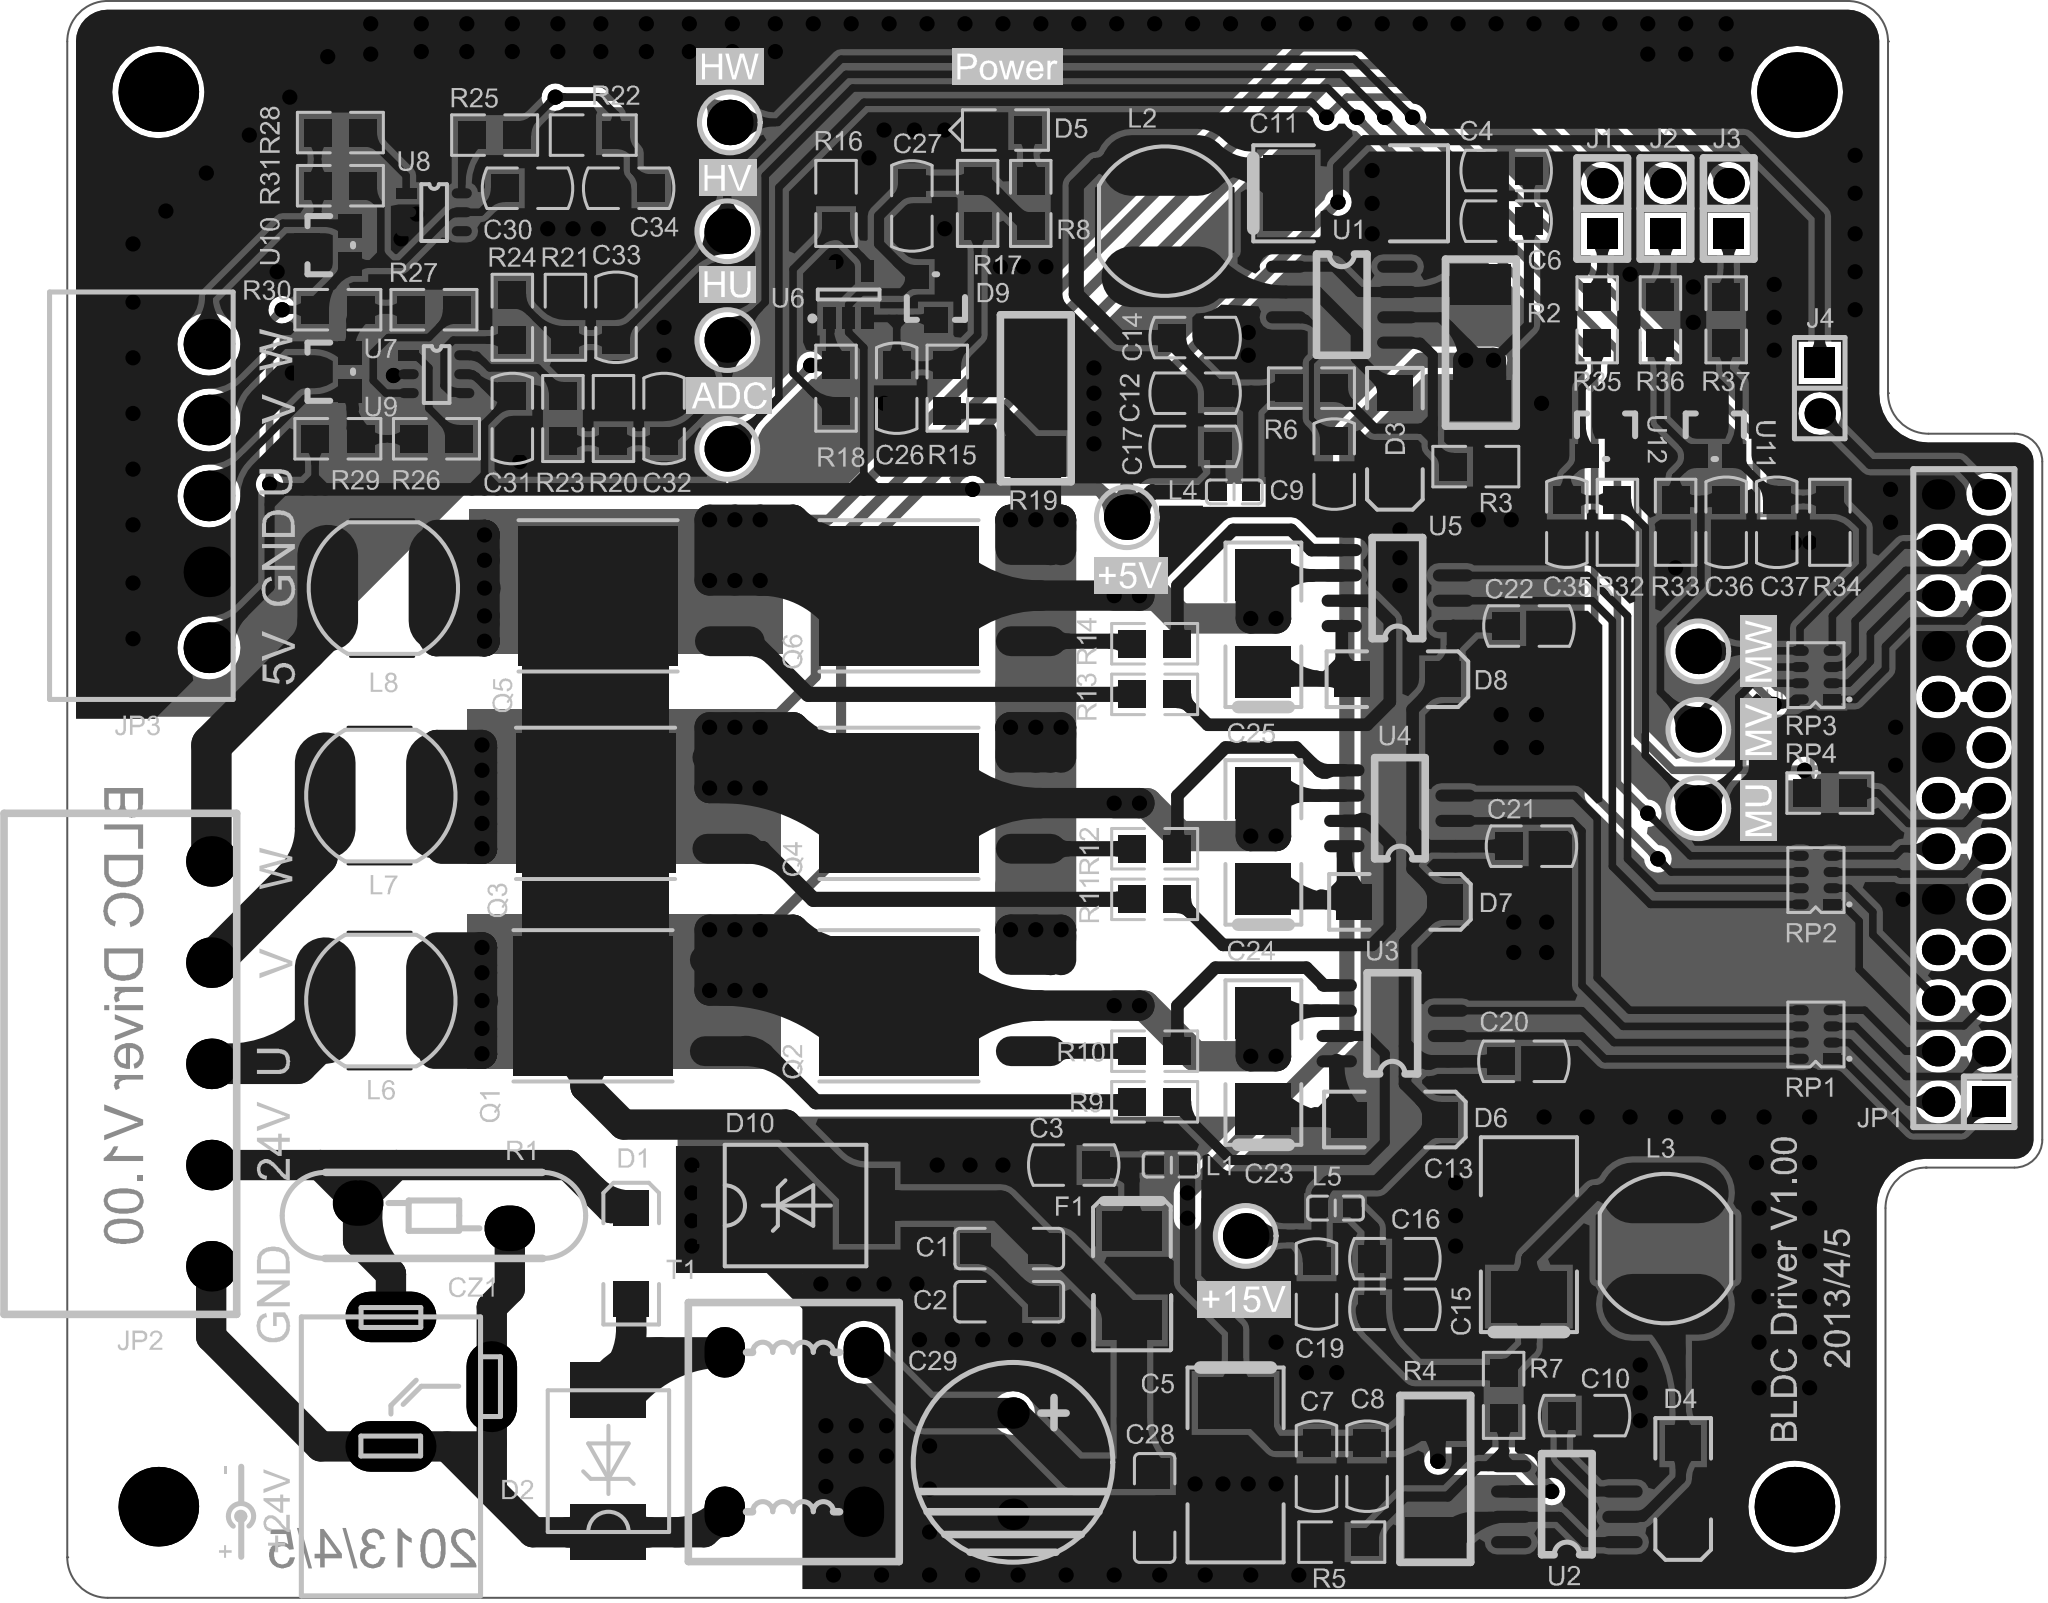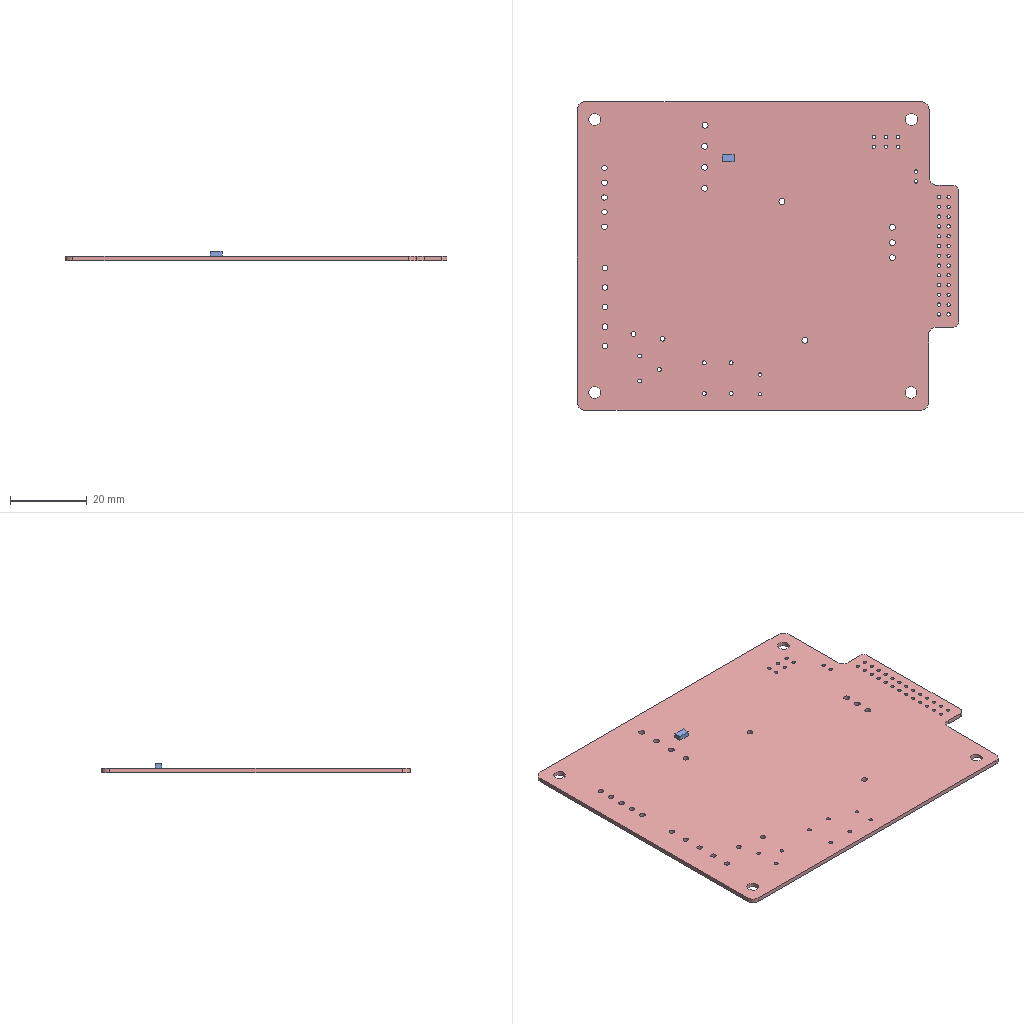Circuit board layout | Altium Designer | box 99.2 x 80.1 x 2.3 mm
Layer stack:
# Altium Designer layer stack of  (unit mm; dielectric type: 0 none, 1 core, 2 prepreg, 3 surface material)
index,name,kind,layer,copper_thickness_mm,dielectric_type,dielectric_thickness_mm,dielectric_material,dielectric_constant
0,Top Paste,other,,,,,,
1,Top Overlay,other,,,,,,
2,Top Solder,dielectric,,,3,0.0102,Solder Resist,3.5
3,Top Layer,copper,Top Layer,0.0356,,,,
4,Dielectric1,dielectric,,,1,0.32,FR-4,4.8
5,GND1,copper,GND1,0.0356,,,,
6,Dielectric2,dielectric,,,2,0.32,FR-4,4.8
7,GND2,copper,GND2,0.0356,,,,
8,Dielectric3,dielectric,,,1,0.32,FR-4,4.8
9,Bottom Layer,copper,Bottom Layer,0.0356,,,,
10,Bottom Solder,dielectric,,,3,0.0102,Solder Resist,3.5
11,Bottom Overlay,other,,,,,,
12,Bottom Paste,other,,,,,,
# drill layer pairs: low layer,high layer
drill_pair,Top Layer,Bottom Layer
Part placement:
Designator,Comment,Layer,Footprint,Center-X(mm),Center-Y(mm),Rotation
J4,CON2,TopLayer,SIP-2,88.011,60.706,270
C1,1nF/2KV,TopLayer,1206C,47.307,17.526,180
C2,1nF/2KV,TopLayer,1206C,47.307,14.859,180
C3,1nF,TopLayer,0805C,50.546,21.717,180
C4,100nF,TopLayer,0805C,72.263,71.628,180
C5,100µF,50V,TopLayer,CAP-D,58.674,6.604,360
C6,1nF,TopLayer,0805C,72.263,69.088,180
C7,100nF,TopLayer,0805C,62.738,6.604,270
C8,1nF,TopLayer,0805C,65.278,6.604,270
C9,2.2nF,TopLayer,0805C,63.627,56.896,270
C10,2.2nF,TopLayer,0805C,76.2,9.144,360
C11,47µF,25V,TopLayer,CAP-D,64.516,70.485,90
C12,100nF,TopLayer,0805C,56.642,60.452,180
C13,100µF,50V,TopLayer,CAP-D,73.406,18.288,180
C14,1nF,TopLayer,0805C,56.642,63.246,360
C15,100nF,TopLayer,0805C,66.675,14.478,360
C16,1nF,TopLayer,0805C,66.675,17.018,360
C17,100pF,TopLayer,0805C,56.642,57.785,180
C19,100pF,TopLayer,0805C,62.738,15.748,270
C20,100nF,TopLayer,0805C,73.152,26.924,180
C21,100nF,TopLayer,0805C,73.533,37.719,180
C22,100nF,TopLayer,0805C,73.406,48.768,180
C23,10uF,25V,TopLayer,CAP-C,60.071,26.924,180
C24,10uF,25V,TopLayer,CAP-C,60.071,37.973,180
C25,10uF,25V,TopLayer,CAP-C,60.071,48.895,180
C26,10nF,TopLayer,0805C,41.656,60.706,90
C27,100nF,TopLayer,0805C,42.418,69.85,90
C28,1nF/2KV,TopLayer,1206C,54.61,4.508,270
C29,330µF,50V,TopLayer,电解电容,47.498,6.731,90
C30,100nF,TopLayer,0805C,23.114,70.739,360
C31,100nF,TopLayer,0805C,22.352,59.182,90
C32,100pF,TopLayer,0805C,29.972,59.182,90
C33,100pF,TopLayer,0805C,27.559,64.262,90
C34,100pF,TopLayer,0805C,28.194,70.739,180
C35,10nF,TopLayer,0805C,75.311,53.975,90
C36,10nF,TopLayer,0805C,83.312,53.975,90
C37,10nF,TopLayer,0805C,85.852,53.975,90
CZ1,POWER,TopLayer,POWER-AC,18.788,10.847,270
D1,SK310A,TopLayer,DO-214AC,28.321,17.272,90
D2,1SMC30AT3,TopLayer,1SMC17AT,27.178,6.858,90
D3,SK310A,TopLayer,DO-214AC,66.675,58.166,270
D4,SK310A,TopLayer,DO-214AC,81.153,5.461,270
D5,Power,TopLayer,0805D,47.117,73.66,180
D6,SK310A,TopLayer,DO-214AC,66.675,24.003,360
D7,SK310A,TopLayer,DO-214AC,66.929,34.925,360
D8,SK310A,TopLayer,DO-214AC,66.802,46.101,360
D9,BAT54S,TopLayer,SOT-23,43.624,65.202,180
D10,1SMC30AT3,TopLayer,1SMC17AT,36.576,19.685,360
F1,SMD050,TopLayer,1812DT,53.467,16.167,270
J1,CON2,TopLayer,SIP-2,77.089,69.723,90
J2,CON2,TopLayer,SIP-2,80.264,69.723,90
J3,CON2,TopLayer,SIP-2,83.439,69.723,90
JP1,HDR13×2,TopLayer,IDC-26,95.25,40.132,90
JP2,CON5,TopLayer,CON-5-5.0,7.239,26.797,90
JP3,CON5,TopLayer,CON-5-3.81,7.112,55.296,90
L1,CBG160808U121T,TopLayer,0603C,55.435,21.717,360
L2,220uH,TopLayer,L-7.5S,55.118,69.088,180
L3,220uH,TopLayer,L-7.5S,80.264,17.526,180
L4,CBG160808U121T,TopLayer,0603C,58.611,55.499,180
L5,CBG160808U121T,TopLayer,0603C,63.691,19.558,180
L6,47uH,TopLayer,L-7.5S,15.748,29.972,270
L7,47uH,TopLayer,L-7.5S,15.748,40.259,270
L8,47uH,TopLayer,L-7.5S,15.875,50.673,270
Q1,NTD32N06,TopLayer,DPAK-3,29.718,29.722,90
Q2,NTD32N06,TopLayer,DPAK-3,45.085,29.722,90
Q3,NTD32N06,TopLayer,DPAK-3,29.845,39.882,90
Q4,NTD32N06,TopLayer,DPAK-3,45.085,39.882,90
Q5,NTD32N06,TopLayer,DPAK-3,29.972,50.296,90
Q6,NTD32N06,TopLayer,DPAK-3,45.085,50.296,90
R1,330KD14,TopLayer,AX-.3/.6,18.415,19.177,90
R2,0.18O,TopLayer,2512,70.993,62.992,90
R3,2.2KO,TopLayer,0805R,70.739,56.769,360
R4,0.18O,TopLayer,2512,68.707,5.969,270
R5,1KO,TopLayer,0805R,64.008,2.794,180
R6,6.8KO,1%,TopLayer,0805R,62.484,60.706,180
R7,11KO,1%,TopLayer,0805R,72.136,10.16,90
R8,2KO,TopLayer,0805R,48.387,69.977,90
R9,33O,TopLayer,0805R,54.61,24.892,180
R10,33O,TopLayer,0805R,54.61,27.432,180
R11,33O,TopLayer,0805R,54.61,35.052,180
R12,33O,TopLayer,0805R,54.61,37.592,180
R13,33O,TopLayer,0805R,54.61,45.339,180
R14,33O,TopLayer,0805R,54.61,47.879,180
R15,1KO,TopLayer,0805R,44.196,60.706,270
R16,150KO,TopLayer,0805R,38.608,69.977,90
R17,20KO,TopLayer,0805R,45.72,69.977,270
R18,300KO,TopLayer,0805R,38.608,60.706,270
R19,0.33O,TopLayer,2512,48.641,60.198,270
R20,10KO,TopLayer,0805R,27.432,59.182,270
R21,10KO,TopLayer,0805R,25.019,64.262,270
R22,10KO,TopLayer,0805R,26.416,73.406,360
R23,6.8KO,TopLayer,0805R,24.892,59.182,90
R24,6.8KO,TopLayer,0805R,22.352,64.262,270
R25,6.8KO,TopLayer,0805R,21.463,73.406,180
R26,33O,TopLayer,0805R,18.542,58.166,180
R27,33O,TopLayer,0805R,18.415,64.643,180
R28,33O,TopLayer,0805R,13.716,73.533,180
R29,4.7KO,TopLayer,0805R,13.589,58.166,180
R30,4.7KO,TopLayer,0805R,13.589,64.643,180
R31,4.7KO,TopLayer,0805R,13.716,70.866,360
R32,10KO,TopLayer,0805R,77.851,53.975,270
R33,10KO,TopLayer,0805R,80.772,53.975,270
R34,10KO,TopLayer,0805R,88.519,53.975,270
R35,100KO,TopLayer,0805R,76.835,64.135,270
R36,100KO,TopLayer,0805R,80.01,64.135,270
R37,100KO,TopLayer,0805R,83.312,64.135,270
RP1,33O,TopLayer,PZ-4-0.8B,87.833,28.27,180
RP2,33O,TopLayer,PZ-4-0.8B,87.833,36.017,180
RP3,33O,TopLayer,PZ-4-0.8B,87.833,46.304,180
RP4,33O,TopLayer,0805R,88.519,40.386,180
T1,Com Tra,TopLayer,L-2-XIAO,36.513,8.319,180
TP2,+5V,TopLayer,PAD(60),53.213,54.229,360
TP4,+15V,TopLayer,PAD(60),59.182,18.161,360
TP5,ADC,TopLayer,PAD(60),33.147,57.658,0
TP6,HU,TopLayer,PAD(60),33.147,63.119,180
TP7,HV,TopLayer,PAD(60),33.147,68.58,180
TP8,HW,TopLayer,PAD(60),33.274,74.041,180
TP9,MU,TopLayer,PAD(60),81.915,39.624,180
TP10,MV,TopLayer,PAD(60),81.915,43.561,270
TP11,MW,TopLayer,PAD(60),81.915,47.498,180
U1,NCP3063,TopLayer,SO-8,64.008,64.897,360
U2,NCP3063,TopLayer,SO-8,75.311,4.699,180
U3,NCP5106B,TopLayer,SO-8,66.548,28.829,180
U4,NCP5106B,TopLayer,SO-8,66.929,39.624,180
U5,NCP5106B,TopLayer,SO-8,66.802,50.673,180
U6,LMC7101QM5,TopLayer,MF05A_N,39.243,65.405,90
U7,SN74LVC2G14DBVR,TopLayer,SOT-23-6,18.542,61.407,360
U8,SN74LVC2G14DBVR,TopLayer,SOT-23-6,18.415,69.535,360
U9,PESD5V2S2UT,TopLayer,SOT-23,13.132,61.532,90
U10,PESD5V2S2UT,TopLayer,SOT-23,13.132,67.882,90
U11,PESD3V3S2UT,TopLayer,SOT-23,82.74,58.369,360
U12,PESD3V3S2UT,TopLayer,SOT-23,77.279,58.369,360
Pad and via stacks:
# Altium Designer via and pad stacks of  (unit mm). Each distinct definition once, with the count of objects using it.
# via: kind,start_layer,end_layer,hole_mm,diameter_mm,mode(0 simple;1 top-mid-bottom;2 full stack),diameter_per_layer,count,example_net
# pad: kind,layer,hole_mm,hole_type(0 round;1 square;2 slot),plating,top_size,top_shape(1 round;2 rect;3 octagon;9 rounded rect),mid_size,bottom_size,mode,footprint,size_per_layer,count,example
pad,Top Layer,0,0,plated,0.889x0.508,1,0.889x0.508,0.889x0.508,0,PZ-4-0.8B,,21,RP3.2
pad,Top Layer,0,0,plated,0.889x0.508,2,0.889x0.508,0.889x0.508,0,PZ-4-0.8B,,3,RP3.1
pad,Top Layer,0,0,plated,1.397x1.397,2,1.397x1.397,1.397x1.397,0,0805R,,68,RP4.2
pad,Top Layer,0,0,plated,1.397x1.397,2,1.397x1.397,1.397x1.397,0,0805D,,2,D5.1
pad,Top Layer,0,0,plated,1.397x1.397,2,1.397x1.397,1.397x1.397,0,0805C,,52,C6.2
pad,Top Layer,0,0,plated,2.6x3.8,2,2.6x3.8,2.6x3.8,0,CAP-D,,6,C11.2
pad,Top Layer,0,0,plated,1.778x1.778,2,1.778x1.778,1.778x1.778,0,DO-214AC,,12,D3.2
pad,Top Layer,0,0,plated,6.35x3.048,1,6.35x3.048,6.35x3.048,0,L-7.5S,,10,L2.1
pad,Top Layer,0,0,plated,0.889x0.889,2,0.889x0.889,0.889x0.889,0,0603C,,6,L4.1
pad,Top Layer,0,0,plated,2.032x3.048,2,2.032x3.048,2.032x3.048,0,2512,,6,R2.2
pad,Top Layer,0,0,plated,2.032x0.6096,1,2.032x0.6096,2.032x0.6096,0,SO-8,,40,U1.1
pad,Top Layer,0,0,plated,2.794x3.81,2,2.794x3.81,2.794x3.81,0,1SMC17AT,,4,D2.1
pad,Top Layer,0,0,plated,1.524x1.524,2,1.524x1.524,1.524x1.524,0,1206C,,6,C2.1
pad,Top Layer,0,0,plated,2x3,2,2x3,2x3,0,1812DT,,2,F1.1
pad,Top Layer,0,0,plated,1.168x1.168,2,1.168x1.168,1.168x1.168,0,SOT-23,,10,D9.1
pad,Top Layer,0,0,plated,1.168x1.27,2,1.168x1.27,1.168x1.27,0,SOT-23,,5,D9.3
pad,Top Layer,0,0,plated,0.65x1.1,2,0.65x1.1,0.65x1.1,0,MF05A_N,,5,U6.5
pad,Top Layer,0,0,plated,2.6x2.8,2,2.6x2.8,2.6x2.8,0,CAP-C,,6,C25.1
pad,Top Layer,0,0,plated,7x8,2,7x8,7x8,0,DPAK-3,,6,Q2.2
pad,Top Layer,0,0,plated,1.5x3.5,1,1.5x3.5,1.5x3.5,0,DPAK-3,,12,Q2.3
pad,Top Layer,0,0,plated,1.016x0.508,2,1.016x0.508,1.016x0.508,0,SOT-23-6,,2,U8.1
pad,Top Layer,0,0,plated,1.016x0.508,1,1.016x0.508,1.016x0.508,0,SOT-23-6,,10,U8.2
pad,Multi-Layer,0.889,0,plated,1.524x1.524,1,1.524x1.524,1.524x1.524,0,SIP-2,,4,J4.2
pad,Multi-Layer,0.889,0,plated,1.524x1.524,2,1.524x1.524,1.524x1.524,0,SIP-2,,4,J4.1
pad,Multi-Layer,3.1,0,plated,4x4,1,4x4,4x4,0,,,4,0
pad,Multi-Layer,0.889,0,plated,1.524x1.676,2,1.524x1.676,1.524x1.676,0,IDC-26,,1,JP1.1
pad,Multi-Layer,0.889,0,plated,1.524x1.676,1,1.524x1.676,1.524x1.676,0,IDC-26,,25,JP1.2
pad,Multi-Layer,1.422,0,plated,2.54x2.54,1,2.54x2.54,2.54x2.54,0,CON-5-5.0,,5,JP2.5
pad,Multi-Layer,1.524,0,plated,2.286x2.286,1,2.286x2.286,2.286x2.286,0,PAD(60),,9,TP2.1
pad,Multi-Layer,1.27,0,plated,2.54x2.286,1,2.54x2.286,2.54x2.286,0,AX-.3/.6,,2,R1.1
pad,Multi-Layer,1.016,0,plated,2.54x2.032,1,2.54x2.032,2.54x2.032,0,L-2-XIAO,,4,T1.1
pad,Multi-Layer,0.889,0,plated,1.575x1.575,1,1.575x1.575,1.575x1.575,0,\u00B5\u00E7\u00BD\u00E2\u00B5\u00E7\u00C8\u00DD,,2,C29.2
pad,Multi-Layer,1.016,0,plated,2.54x4.572,1,2.54x4.572,2.54x4.572,0,POWER-AC,,1,CZ1.1
pad,Multi-Layer,1.016,0,plated,4.572x2.54,1,4.572x2.54,4.572x2.54,0,POWER-AC,,2,CZ1.3
pad,Multi-Layer,1.422,0,plated,2.54x2.54,1,2.54x2.54,2.54x2.54,0,CON-5-3.81,,5,JP3.5
via,Top Layer,Bottom Layer,0.508,0.762,0,,268,GND
Copper pours:
name,layer,net,type(0 solid;1 hatched;2 none)
Top Layer-No Net,Bottom Layer,GND,0
Top Layer-No Net 1,Top Layer,GND,0
Design rules, without the lines most boards share:
# Altium Designer design rules of  (exported by Altium Designer, unit mm)
# columns: name | kind | enabled | priority | scope1 | scope2 | descriptor | typed fields (field=value)
Clearance | 0 | enabled | 1 | All | All | Clearance Constraint (Gap=12mil) (All),(All) | gap=0.3048
PlaneConnect | 6 | enabled | 1 | All | All | Power Plane Connect Rule(Relief Connect )(Expansion=20mil) (Conductor Width=10mil) (Air Gap=10mil) (Entries=4) (All) | relief_conductor_width=0.254 relief_entries=4 relief_expansion=0.508
PolygonConnect | 20 | enabled | 2 | All | All | Polygon Connect Rule(Direct Connect )(Conductor Width=10mil) (Relief Angle=90 Angle) (Entries=4) (Air Gap Width=10mil) (All),(All) | connect_style(0=relief,1=direct,2=none)=1 relief_conductor_width=0.254 relief_entries=4
Width | 2 | enabled | 3 | All | All | Width Constraint (Min=10mil) (Max=200mil) (Preferred=15mil) (All) |
RoutingVias | 11 | enabled | 1 | All | All | Routing Via (MinHoleWidth=16mil) (MaxHoleWidth=20mil) (PreferredHoleWidth=20mil) (MinWidth=20mil) (MaxWidth=30mil) (PreferedWidth=30mil) (All) | via_min_hole=0.4064 via_max_hole=0.508 via_preferred_diameter=0.762 via_preferred_hole=0.508
SolderMaskExpansion | 13 | enabled | 1 | All | All | Solder Mask Expansion (Expansion =4mil) (All) | expansion=0.1016
HoleSize | 42 | enabled | 1 | All | All | Hole Size Constraint (Min=1mil) (Max=260mil) (All) |
DiffPairsRouting | 51 | enabled | 1 | All | All | Differential Pairs Uncoupled Length using the Gap Constraints (Min=10mil) (Max=10mil) (Prefered=10mil)  and Width Constraints (Min=15mil) (Max=15mil) (Prefered=15mil) (All) |
HoleToHoleClearance | 52 | enabled | 1 | All | All | Hole To Hole Clearance (Gap=7mil) (All),(All) | gap=0.1778
MinimumSolderMaskSliver | 53 | enabled | 1 | All | All | Minimum Solder Mask Sliver (Gap=5mil) (All),(All) |
SilkscreenOverComponentPads | 54 | disabled | 1 | IsPad | All | Silk To Solder Mask (Clearance=0mil) (Disabled)(IsPad),(All) |
SilkToSilkClearance | 55 | disabled | 1 | All | All | Silk to Silk (Clearance=5mil) (Disabled)(All),(All) |
+24V | 2 | enabled | 2 | InNet('+24V') | All | Width Constraint (Min=20mil) (Max=100mil) (Preferred=40mil) (InNet('+24V')) |
GND | 2 | enabled | 1 | InNet('GND') | All | Width Constraint (Min=8mil) (Max=60mil) (Preferred=10mil) (InNet('GND')) |
VIA | 20 | enabled | 1 | All | All | Polygon Connect Rule(Direct Connect )(Conductor Width=10mil) (Relief Angle=90 Angle) (Entries=4) (Air Gap Width=10mil) (All),(All) | connect_style(0=relief,1=direct,2=none)=1 relief_conductor_width=0.254 relief_entries=4
Classes set for this board:
# Altium Designer classes of  (member kind: 0 net, 1 component, 2 from-to, 3 pad, 4 layer, 5 differential pair, 6 design channel, 7 polygon, 8 structure, 9 xSignal)
# columns: class name | member kind | superclass | members
U_02 | 1 | no | C1; C2; C3; C4; C5; C6; C7; C8; C9; C10; C11; C12; C13; C14; C15; C16; C17; C19; D1; D2; D3; D4; D5; F1; L1; L2; L3; L4; L5; R1; R2; R3; R4; R5; R6; R7; R8; T1; TP2; TP4; U1; U2;
U_03 | 1 | no | C20; C21; C22; C23; C24; C25; C26; C27; C28; C29; D6; D7; D8; D9; D10; L6; L7; L8; Q1; Q2; Q3; Q4; Q5; Q6; R9; R10; R11; R12; R13; R14; R15; R16; R17; R18; R19; TP5; U3; U4; U5; U6;
U_04 | 1 | no | C30; C31; C32; C33; C34; R20; R21; R22; R23; R24; R25; R26; R27; R28; R29; R30; R31; TP6; TP7; TP8; U7; U8; U9; U10;
U_05 | 1 | no | C35; C36; C37; J1; J2; J3; R32; R33; R34; R35; R36; R37; TP9; TP10; TP11; U11; U12;
Components Class 1 | 1 | no | U5; U4; U3; R14; R13; R12; R11; R10; R9; D8; D7; D6; C25; C24; C23; C22; C21; C20;
Components Class 2 | 1 | no | U1; R6; R3; L4; L2; D3; C17; C14; C12; C11; C9; C6; C4;